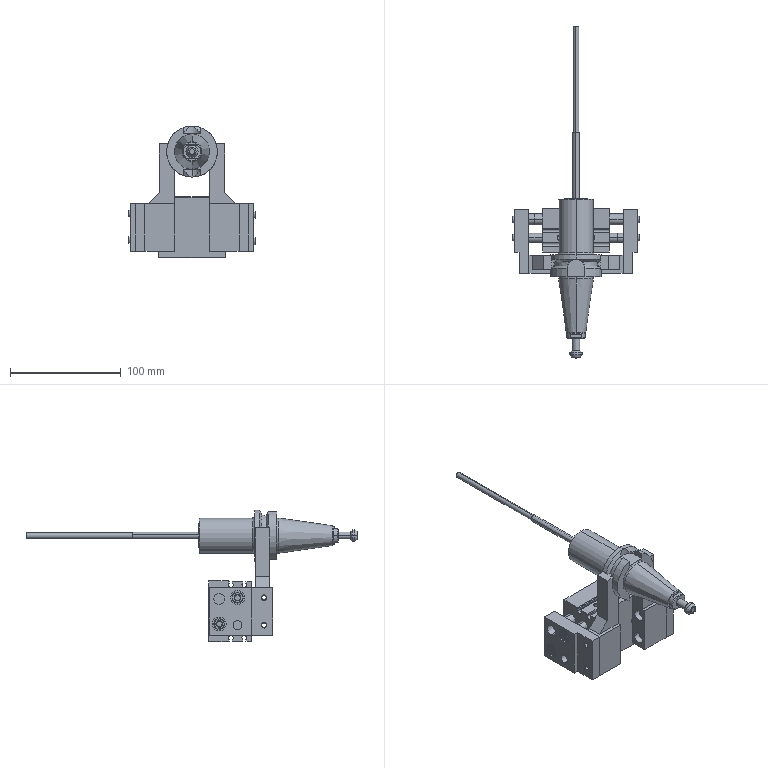Part | SolidWorks | features MirrorCompFeat 1, ReferencePattern 1 | 17 solids | 426 faces | box 115 x 300 x 119 mm | volume 333803 mm3 | cylinder 174 | plane 171 | cone 65 | torus 16 | commonest cylinder face diameters 10 x28 4.134 x24 6 x14 5.5 x12 8 x12 3 x11